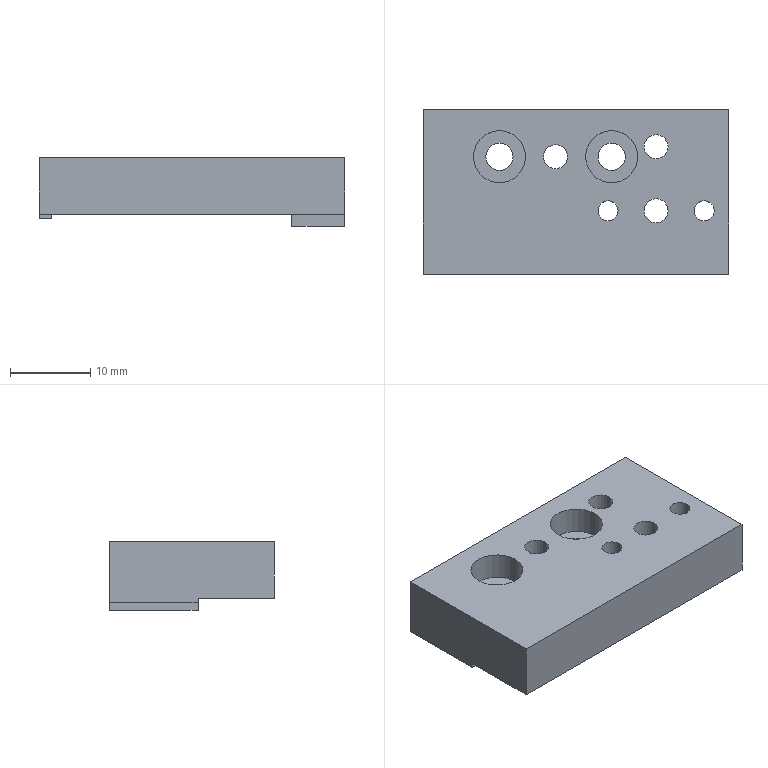Part | STEP file | 11-FG-E02711 | 1 solid | 32 faces | box 38.1 x 20.5 x 8.5 mm | volume 5078 mm3 | cylinder 18 | plane 14 | commonest cylinder face diameters 3 x6 2.5 x4 3.4 x4 6.5 x4
STEP:
#1=CARTESIAN_POINT('',(14.05,8.4,0.));
#2=VERTEX_POINT('',#1);
#3=CARTESIAN_POINT('',(11.05,8.4,0.));
#4=VERTEX_POINT('',#3);
#5=CARTESIAN_POINT('',(12.55,8.4,0.));
#6=DIRECTION('',(0.,0.,-1.));
#7=DIRECTION('',(-1.,0.,0.));
#8=AXIS2_PLACEMENT_3D('',#5,#6,#7);
#9=CIRCLE('',#8,1.5);
#10=EDGE_CURVE('',#2,#4,#9,.T.);
#11=ORIENTED_EDGE('',*,*,#10,.T.);
#12=CARTESIAN_POINT('',(11.05,8.4,7.));
#13=VERTEX_POINT('',#12);
#14=CARTESIAN_POINT('',(11.05,8.4,7.));
#15=DIRECTION('',(0.,0.,1.));
#16=VECTOR('',#15,1000.);
#17=LINE('',#14,#16);
#18=EDGE_CURVE('',#4,#13,#17,.T.);
#19=ORIENTED_EDGE('',*,*,#18,.T.);
#20=CARTESIAN_POINT('',(14.05,8.4,7.));
#21=VERTEX_POINT('',#20);
#22=CARTESIAN_POINT('',(12.55,8.4,7.));
#23=DIRECTION('',(0.,0.,1.));
#24=DIRECTION('',(1.,0.,0.));
#25=AXIS2_PLACEMENT_3D('',#22,#23,#24);
#26=CIRCLE('',#25,1.5);
#27=EDGE_CURVE('',#13,#21,#26,.T.);
#28=ORIENTED_EDGE('',*,*,#27,.T.);
#29=CARTESIAN_POINT('',(14.05,8.4,7.));
#30=DIRECTION('',(0.,0.,1.));
#31=VECTOR('',#30,1000.);
#32=LINE('',#29,#31);
#33=EDGE_CURVE('',#2,#21,#32,.T.);
#34=ORIENTED_EDGE('',*,*,#33,.F.);
#35=EDGE_LOOP('',(#11,#19,#28,#34));
#36=FACE_OUTER_BOUND('',#35,.T.);
#37=CARTESIAN_POINT('',(12.55,8.4,7.));
#38=DIRECTION('',(0.,0.,1.));
#39=DIRECTION('',(1.,0.,0.));
#40=AXIS2_PLACEMENT_3D('',#37,#38,#39);
#41=CYLINDRICAL_SURFACE('',#40,1.5);
#42=ADVANCED_FACE('',(#36),#41,.F.);
#43=CARTESIAN_POINT('',(14.05,16.4,0.));
#44=VERTEX_POINT('',#43);
#45=CARTESIAN_POINT('',(11.05,16.4,0.));
#46=VERTEX_POINT('',#45);
#47=CARTESIAN_POINT('',(12.55,16.4,0.));
#48=DIRECTION('',(0.,0.,-1.));
#49=DIRECTION('',(-1.,0.,0.));
#50=AXIS2_PLACEMENT_3D('',#47,#48,#49);
#51=CIRCLE('',#50,1.5);
#52=EDGE_CURVE('',#44,#46,#51,.T.);
#53=ORIENTED_EDGE('',*,*,#52,.T.);
#54=CARTESIAN_POINT('',(11.05,16.4,7.));
#55=VERTEX_POINT('',#54);
#56=CARTESIAN_POINT('',(11.05,16.4,7.));
#57=DIRECTION('',(0.,0.,1.));
#58=VECTOR('',#57,1000.);
#59=LINE('',#56,#58);
#60=EDGE_CURVE('',#46,#55,#59,.T.);
#61=ORIENTED_EDGE('',*,*,#60,.T.);
#62=CARTESIAN_POINT('',(14.05,16.4,7.));
#63=VERTEX_POINT('',#62);
#64=CARTESIAN_POINT('',(12.55,16.4,7.));
#65=DIRECTION('',(0.,0.,1.));
#66=DIRECTION('',(1.,0.,0.));
#67=AXIS2_PLACEMENT_3D('',#64,#65,#66);
#68=CIRCLE('',#67,1.5);
#69=EDGE_CURVE('',#55,#63,#68,.T.);
#70=ORIENTED_EDGE('',*,*,#69,.T.);
#71=CARTESIAN_POINT('',(14.05,16.4,7.));
#72=DIRECTION('',(0.,0.,1.));
#73=VECTOR('',#72,1000.);
#74=LINE('',#71,#73);
#75=EDGE_CURVE('',#44,#63,#74,.T.);
#76=ORIENTED_EDGE('',*,*,#75,.F.);
#77=EDGE_LOOP('',(#53,#61,#70,#76));
#78=FACE_OUTER_BOUND('',#77,.T.);
#79=CARTESIAN_POINT('',(12.55,16.4,7.));
#80=DIRECTION('',(0.,0.,1.));
#81=DIRECTION('',(1.,0.,0.));
#82=AXIS2_PLACEMENT_3D('',#79,#80,#81);
#83=CYLINDRICAL_SURFACE('',#82,1.5);
#84=ADVANCED_FACE('',(#78),#83,.F.);
#85=CARTESIAN_POINT('',(-1.5,15.147,0.));
#86=VERTEX_POINT('',#85);
#87=CARTESIAN_POINT('',(1.5,15.147,0.));
#88=VERTEX_POINT('',#87);
#89=CARTESIAN_POINT('',(0.,15.147,0.));
#90=DIRECTION('',(0.,0.,1.));
#91=DIRECTION('',(1.,0.,0.));
#92=AXIS2_PLACEMENT_3D('',#89,#90,#91);
#93=CIRCLE('',#92,1.5);
#94=EDGE_CURVE('',#86,#88,#93,.T.);
#95=ORIENTED_EDGE('',*,*,#94,.F.);
#96=CARTESIAN_POINT('',(-1.5,15.147,7.));
#97=VERTEX_POINT('',#96);
#98=CARTESIAN_POINT('',(-1.5,15.147,7.));
#99=DIRECTION('',(0.,0.,1.));
#100=VECTOR('',#99,1000.);
#101=LINE('',#98,#100);
#102=EDGE_CURVE('',#86,#97,#101,.T.);
#103=ORIENTED_EDGE('',*,*,#102,.T.);
#104=CARTESIAN_POINT('',(1.5,15.147,7.));
#105=VERTEX_POINT('',#104);
#106=CARTESIAN_POINT('',(0.,15.147,7.));
#107=DIRECTION('',(0.,0.,1.));
#108=DIRECTION('',(1.,0.,0.));
#109=AXIS2_PLACEMENT_3D('',#106,#107,#108);
#110=CIRCLE('',#109,1.5);
#111=EDGE_CURVE('',#97,#105,#110,.T.);
#112=ORIENTED_EDGE('',*,*,#111,.T.);
#113=CARTESIAN_POINT('',(1.5,15.147,7.));
#114=DIRECTION('',(0.,0.,1.));
#115=VECTOR('',#114,1000.);
#116=LINE('',#113,#115);
#117=EDGE_CURVE('',#88,#105,#116,.T.);
#118=ORIENTED_EDGE('',*,*,#117,.F.);
#119=EDGE_LOOP('',(#95,#103,#112,#118));
#120=FACE_OUTER_BOUND('',#119,.T.);
#121=CARTESIAN_POINT('',(0.,15.147,7.));
#122=DIRECTION('',(0.,0.,1.));
#123=DIRECTION('',(1.,0.,0.));
#124=AXIS2_PLACEMENT_3D('',#121,#122,#123);
#125=CYLINDRICAL_SURFACE('',#124,1.5);
#126=ADVANCED_FACE('',(#120),#125,.F.);
#127=CARTESIAN_POINT('',(-10.25,15.147,3.6));
#128=VERTEX_POINT('',#127);
#129=CARTESIAN_POINT('',(-3.75,15.147,3.6));
#130=VERTEX_POINT('',#129);
#131=CARTESIAN_POINT('',(-7.,15.147,3.6));
#132=DIRECTION('',(0.,0.,1.));
#133=DIRECTION('',(1.,0.,0.));
#134=AXIS2_PLACEMENT_3D('',#131,#132,#133);
#135=CIRCLE('',#134,3.25);
#136=EDGE_CURVE('',#128,#130,#135,.T.);
#137=ORIENTED_EDGE('',*,*,#136,.F.);
#138=CARTESIAN_POINT('',(-10.25,15.147,7.));
#139=VERTEX_POINT('',#138);
#140=CARTESIAN_POINT('',(-10.25,15.147,7.));
#141=DIRECTION('',(0.,0.,1.));
#142=VECTOR('',#141,1000.);
#143=LINE('',#140,#142);
#144=EDGE_CURVE('',#128,#139,#143,.T.);
#145=ORIENTED_EDGE('',*,*,#144,.T.);
#146=CARTESIAN_POINT('',(-3.75,15.147,7.));
#147=VERTEX_POINT('',#146);
#148=CARTESIAN_POINT('',(-7.,15.147,7.));
#149=DIRECTION('',(0.,0.,1.));
#150=DIRECTION('',(1.,0.,0.));
#151=AXIS2_PLACEMENT_3D('',#148,#149,#150);
#152=CIRCLE('',#151,3.25);
#153=EDGE_CURVE('',#139,#147,#152,.T.);
#154=ORIENTED_EDGE('',*,*,#153,.T.);
#155=CARTESIAN_POINT('',(-3.75,15.147,7.));
#156=DIRECTION('',(0.,0.,1.));
#157=VECTOR('',#156,1000.);
#158=LINE('',#155,#157);
#159=EDGE_CURVE('',#130,#147,#158,.T.);
#160=ORIENTED_EDGE('',*,*,#159,.F.);
#161=EDGE_LOOP('',(#137,#145,#154,#160));
#162=FACE_OUTER_BOUND('',#161,.T.);
#163=CARTESIAN_POINT('',(-7.,15.147,7.));
#164=DIRECTION('',(0.,0.,1.));
#165=DIRECTION('',(1.,0.,0.));
#166=AXIS2_PLACEMENT_3D('',#163,#164,#165);
#167=CYLINDRICAL_SURFACE('',#166,3.25);
#168=ADVANCED_FACE('',(#162),#167,.F.);
#169=CARTESIAN_POINT('',(-8.7,15.147,0.));
#170=VERTEX_POINT('',#169);
#171=CARTESIAN_POINT('',(-5.3,15.147,0.));
#172=VERTEX_POINT('',#171);
#173=CARTESIAN_POINT('',(-7.,15.147,0.));
#174=DIRECTION('',(0.,0.,1.));
#175=DIRECTION('',(1.,0.,0.));
#176=AXIS2_PLACEMENT_3D('',#173,#174,#175);
#177=CIRCLE('',#176,1.7);
#178=EDGE_CURVE('',#170,#172,#177,.T.);
#179=ORIENTED_EDGE('',*,*,#178,.F.);
#180=CARTESIAN_POINT('',(-8.7,15.147,3.6));
#181=VERTEX_POINT('',#180);
#182=CARTESIAN_POINT('',(-8.7,15.147,7.));
#183=DIRECTION('',(0.,0.,1.));
#184=VECTOR('',#183,1000.);
#185=LINE('',#182,#184);
#186=EDGE_CURVE('',#170,#181,#185,.T.);
#187=ORIENTED_EDGE('',*,*,#186,.T.);
#188=CARTESIAN_POINT('',(-5.3,15.147,3.6));
#189=VERTEX_POINT('',#188);
#190=CARTESIAN_POINT('',(-7.,15.147,3.6));
#191=DIRECTION('',(0.,0.,1.));
#192=DIRECTION('',(1.,0.,0.));
#193=AXIS2_PLACEMENT_3D('',#190,#191,#192);
#194=CIRCLE('',#193,1.7);
#195=EDGE_CURVE('',#181,#189,#194,.T.);
#196=ORIENTED_EDGE('',*,*,#195,.T.);
#197=CARTESIAN_POINT('',(-5.3,15.147,7.));
#198=DIRECTION('',(0.,0.,1.));
#199=VECTOR('',#198,1000.);
#200=LINE('',#197,#199);
#201=EDGE_CURVE('',#172,#189,#200,.T.);
#202=ORIENTED_EDGE('',*,*,#201,.F.);
#203=EDGE_LOOP('',(#179,#187,#196,#202));
#204=FACE_OUTER_BOUND('',#203,.T.);
#205=CARTESIAN_POINT('',(-7.,15.147,7.));
#206=DIRECTION('',(0.,0.,1.));
#207=DIRECTION('',(1.,0.,0.));
#208=AXIS2_PLACEMENT_3D('',#205,#206,#207);
#209=CYLINDRICAL_SURFACE('',#208,1.7);
#210=ADVANCED_FACE('',(#204),#209,.F.);
#211=CARTESIAN_POINT('',(3.75,15.147,3.6));
#212=VERTEX_POINT('',#211);
#213=CARTESIAN_POINT('',(10.25,15.147,3.6));
#214=VERTEX_POINT('',#213);
#215=CARTESIAN_POINT('',(7.,15.147,3.6));
#216=DIRECTION('',(0.,0.,1.));
#217=DIRECTION('',(1.,0.,0.));
#218=AXIS2_PLACEMENT_3D('',#215,#216,#217);
#219=CIRCLE('',#218,3.25);
#220=EDGE_CURVE('',#212,#214,#219,.T.);
#221=ORIENTED_EDGE('',*,*,#220,.F.);
#222=CARTESIAN_POINT('',(3.75,15.147,7.));
#223=VERTEX_POINT('',#222);
#224=CARTESIAN_POINT('',(3.75,15.147,7.));
#225=DIRECTION('',(0.,0.,1.));
#226=VECTOR('',#225,1000.);
#227=LINE('',#224,#226);
#228=EDGE_CURVE('',#212,#223,#227,.T.);
#229=ORIENTED_EDGE('',*,*,#228,.T.);
#230=CARTESIAN_POINT('',(10.25,15.147,7.));
#231=VERTEX_POINT('',#230);
#232=CARTESIAN_POINT('',(7.,15.147,7.));
#233=DIRECTION('',(0.,0.,1.));
#234=DIRECTION('',(1.,0.,0.));
#235=AXIS2_PLACEMENT_3D('',#232,#233,#234);
#236=CIRCLE('',#235,3.25);
#237=EDGE_CURVE('',#223,#231,#236,.T.);
#238=ORIENTED_EDGE('',*,*,#237,.T.);
#239=CARTESIAN_POINT('',(10.25,15.147,7.));
#240=DIRECTION('',(0.,0.,1.));
#241=VECTOR('',#240,1000.);
#242=LINE('',#239,#241);
#243=EDGE_CURVE('',#214,#231,#242,.T.);
#244=ORIENTED_EDGE('',*,*,#243,.F.);
#245=EDGE_LOOP('',(#221,#229,#238,#244));
#246=FACE_OUTER_BOUND('',#245,.T.);
#247=CARTESIAN_POINT('',(7.,15.147,7.));
#248=DIRECTION('',(0.,0.,1.));
#249=DIRECTION('',(1.,0.,0.));
#250=AXIS2_PLACEMENT_3D('',#247,#248,#249);
#251=CYLINDRICAL_SURFACE('',#250,3.25);
#252=ADVANCED_FACE('',(#246),#251,.F.);
#253=CARTESIAN_POINT('',(5.3,15.147,0.));
#254=VERTEX_POINT('',#253);
#255=CARTESIAN_POINT('',(8.7,15.147,0.));
#256=VERTEX_POINT('',#255);
#257=CARTESIAN_POINT('',(7.,15.147,0.));
#258=DIRECTION('',(0.,0.,1.));
#259=DIRECTION('',(1.,0.,0.));
#260=AXIS2_PLACEMENT_3D('',#257,#258,#259);
#261=CIRCLE('',#260,1.7);
#262=EDGE_CURVE('',#254,#256,#261,.T.);
#263=ORIENTED_EDGE('',*,*,#262,.F.);
#264=CARTESIAN_POINT('',(5.3,15.147,3.6));
#265=VERTEX_POINT('',#264);
#266=CARTESIAN_POINT('',(5.3,15.147,7.));
#267=DIRECTION('',(0.,0.,1.));
#268=VECTOR('',#267,1000.);
#269=LINE('',#266,#268);
#270=EDGE_CURVE('',#254,#265,#269,.T.);
#271=ORIENTED_EDGE('',*,*,#270,.T.);
#272=CARTESIAN_POINT('',(8.7,15.147,3.6));
#273=VERTEX_POINT('',#272);
#274=CARTESIAN_POINT('',(7.,15.147,3.6));
#275=DIRECTION('',(0.,0.,1.));
#276=DIRECTION('',(1.,0.,0.));
#277=AXIS2_PLACEMENT_3D('',#274,#275,#276);
#278=CIRCLE('',#277,1.7);
#279=EDGE_CURVE('',#265,#273,#278,.T.);
#280=ORIENTED_EDGE('',*,*,#279,.T.);
#281=CARTESIAN_POINT('',(8.7,15.147,7.));
#282=DIRECTION('',(0.,0.,1.));
#283=VECTOR('',#282,1000.);
#284=LINE('',#281,#283);
#285=EDGE_CURVE('',#256,#273,#284,.T.);
#286=ORIENTED_EDGE('',*,*,#285,.F.);
#287=EDGE_LOOP('',(#263,#271,#280,#286));
#288=FACE_OUTER_BOUND('',#287,.T.);
#289=CARTESIAN_POINT('',(7.,15.147,7.));
#290=DIRECTION('',(0.,0.,1.));
#291=DIRECTION('',(1.,0.,0.));
#292=AXIS2_PLACEMENT_3D('',#289,#290,#291);
#293=CYLINDRICAL_SURFACE('',#292,1.7);
#294=ADVANCED_FACE('',(#288),#293,.F.);
#295=CARTESIAN_POINT('',(5.3,8.4,0.));
#296=VERTEX_POINT('',#295);
#297=CARTESIAN_POINT('',(7.8,8.4,0.));
#298=VERTEX_POINT('',#297);
#299=CARTESIAN_POINT('',(6.55,8.4,0.));
#300=DIRECTION('',(0.,0.,1.));
#301=DIRECTION('',(1.,0.,0.));
#302=AXIS2_PLACEMENT_3D('',#299,#300,#301);
#303=CIRCLE('',#302,1.25);
#304=EDGE_CURVE('',#296,#298,#303,.T.);
#305=ORIENTED_EDGE('',*,*,#304,.F.);
#306=CARTESIAN_POINT('',(5.3,8.4,7.));
#307=VERTEX_POINT('',#306);
#308=CARTESIAN_POINT('',(5.3,8.4,7.));
#309=DIRECTION('',(0.,0.,1.));
#310=VECTOR('',#309,1000.);
#311=LINE('',#308,#310);
#312=EDGE_CURVE('',#296,#307,#311,.T.);
#313=ORIENTED_EDGE('',*,*,#312,.T.);
#314=CARTESIAN_POINT('',(7.8,8.4,7.));
#315=VERTEX_POINT('',#314);
#316=CARTESIAN_POINT('',(6.55,8.4,7.));
#317=DIRECTION('',(0.,0.,1.));
#318=DIRECTION('',(1.,0.,0.));
#319=AXIS2_PLACEMENT_3D('',#316,#317,#318);
#320=CIRCLE('',#319,1.25);
#321=EDGE_CURVE('',#307,#315,#320,.T.);
#322=ORIENTED_EDGE('',*,*,#321,.T.);
#323=CARTESIAN_POINT('',(7.8,8.4,7.));
#324=DIRECTION('',(0.,0.,1.));
#325=VECTOR('',#324,1000.);
#326=LINE('',#323,#325);
#327=EDGE_CURVE('',#298,#315,#326,.T.);
#328=ORIENTED_EDGE('',*,*,#327,.F.);
#329=EDGE_LOOP('',(#305,#313,#322,#328));
#330=FACE_OUTER_BOUND('',#329,.T.);
#331=CARTESIAN_POINT('',(6.55,8.4,7.));
#332=DIRECTION('',(0.,0.,1.));
#333=DIRECTION('',(1.,0.,0.));
#334=AXIS2_PLACEMENT_3D('',#331,#332,#333);
#335=CYLINDRICAL_SURFACE('',#334,1.25);
#336=ADVANCED_FACE('',(#330),#335,.F.);
#337=CARTESIAN_POINT('',(17.3,8.4,0.));
#338=VERTEX_POINT('',#337);
#339=CARTESIAN_POINT('',(19.8,8.4,0.));
#340=VERTEX_POINT('',#339);
#341=CARTESIAN_POINT('',(18.55,8.4,0.));
#342=DIRECTION('',(0.,0.,1.));
#343=DIRECTION('',(1.,0.,0.));
#344=AXIS2_PLACEMENT_3D('',#341,#342,#343);
#345=CIRCLE('',#344,1.25);
#346=EDGE_CURVE('',#338,#340,#345,.T.);
#347=ORIENTED_EDGE('',*,*,#346,.F.);
#348=CARTESIAN_POINT('',(17.3,8.4,7.));
#349=VERTEX_POINT('',#348);
#350=CARTESIAN_POINT('',(17.3,8.4,7.));
#351=DIRECTION('',(0.,0.,1.));
#352=VECTOR('',#351,1000.);
#353=LINE('',#350,#352);
#354=EDGE_CURVE('',#338,#349,#353,.T.);
#355=ORIENTED_EDGE('',*,*,#354,.T.);
#356=CARTESIAN_POINT('',(19.8,8.4,7.));
#357=VERTEX_POINT('',#356);
#358=CARTESIAN_POINT('',(18.55,8.4,7.));
#359=DIRECTION('',(0.,0.,1.));
#360=DIRECTION('',(1.,0.,0.));
#361=AXIS2_PLACEMENT_3D('',#358,#359,#360);
#362=CIRCLE('',#361,1.25);
#363=EDGE_CURVE('',#349,#357,#362,.T.);
#364=ORIENTED_EDGE('',*,*,#363,.T.);
#365=CARTESIAN_POINT('',(19.8,8.4,7.));
#366=DIRECTION('',(0.,0.,1.));
#367=VECTOR('',#366,1000.);
#368=LINE('',#365,#367);
#369=EDGE_CURVE('',#340,#357,#368,.T.);
#370=ORIENTED_EDGE('',*,*,#369,.F.);
#371=EDGE_LOOP('',(#347,#355,#364,#370));
#372=FACE_OUTER_BOUND('',#371,.T.);
#373=CARTESIAN_POINT('',(18.55,8.4,7.));
#374=DIRECTION('',(0.,0.,1.));
#375=DIRECTION('',(1.,0.,0.));
#376=AXIS2_PLACEMENT_3D('',#373,#374,#375);
#377=CYLINDRICAL_SURFACE('',#376,1.25);
#378=ADVANCED_FACE('',(#372),#377,.F.);
#379=CARTESIAN_POINT('',(-16.5,10.,0.));
#380=VERTEX_POINT('',#379);
#381=CARTESIAN_POINT('',(-16.5,0.5,0.));
#382=VERTEX_POINT('',#381);
#383=CARTESIAN_POINT('',(-16.5,0.,0.));
#384=DIRECTION('',(0.,-1.,0.));
#385=VECTOR('',#384,1000.);
#386=LINE('',#383,#385);
#387=EDGE_CURVE('',#380,#382,#386,.T.);
#388=ORIENTED_EDGE('',*,*,#387,.F.);
#389=CARTESIAN_POINT('',(-15.,10.,0.));
#390=VERTEX_POINT('',#389);
#391=CARTESIAN_POINT('',(-23.4,10.,0.));
#392=DIRECTION('',(-1.,0.,0.));
#393=VECTOR('',#392,1000.);
#394=LINE('',#391,#393);
#395=EDGE_CURVE('',#390,#380,#394,.T.);
#396=ORIENTED_EDGE('',*,*,#395,.F.);
#397=CARTESIAN_POINT('',(-15.,21.,0.));
#398=VERTEX_POINT('',#397);
#399=CARTESIAN_POINT('',(-15.,21.,0.));
#400=DIRECTION('',(0.,-1.,0.));
#401=VECTOR('',#400,1000.);
#402=LINE('',#399,#401);
#403=EDGE_CURVE('',#398,#390,#402,.T.);
#404=ORIENTED_EDGE('',*,*,#403,.F.);
#405=CARTESIAN_POINT('',(15.,21.,0.));
#406=VERTEX_POINT('',#405);
#407=CARTESIAN_POINT('',(-27.5,21.,0.));
#408=DIRECTION('',(-1.,0.,0.));
#409=VECTOR('',#408,1000.);
#410=LINE('',#407,#409);
#411=EDGE_CURVE('',#406,#398,#410,.T.);
#412=ORIENTED_EDGE('',*,*,#411,.F.);
#413=CARTESIAN_POINT('',(15.,10.,0.));
#414=VERTEX_POINT('',#413);
#415=CARTESIAN_POINT('',(15.,10.,0.));
#416=DIRECTION('',(0.,1.,0.));
#417=VECTOR('',#416,1000.);
#418=LINE('',#415,#417);
#419=EDGE_CURVE('',#414,#406,#418,.T.);
#420=ORIENTED_EDGE('',*,*,#419,.F.);
#421=CARTESIAN_POINT('',(21.6,10.,0.));
#422=VERTEX_POINT('',#421);
#423=CARTESIAN_POINT('',(21.6,10.,0.));
#424=DIRECTION('',(-1.,0.,0.));
#425=VECTOR('',#424,1000.);
#426=LINE('',#423,#425);
#427=EDGE_CURVE('',#422,#414,#426,.T.);
#428=ORIENTED_EDGE('',*,*,#427,.F.);
#429=CARTESIAN_POINT('',(21.6,0.5,0.));
#430=VERTEX_POINT('',#429);
#431=CARTESIAN_POINT('',(21.6,0.,0.));
#432=DIRECTION('',(0.,1.,0.));
#433=VECTOR('',#432,1000.);
#434=LINE('',#431,#433);
#435=EDGE_CURVE('',#430,#422,#434,.T.);
#436=ORIENTED_EDGE('',*,*,#435,.F.);
#437=CARTESIAN_POINT('',(0.,0.5,0.));
#438=DIRECTION('',(1.,0.,0.));
#439=VECTOR('',#438,1000.);
#440=LINE('',#437,#439);
#441=EDGE_CURVE('',#382,#430,#440,.T.);
#442=ORIENTED_EDGE('',*,*,#441,.F.);
#443=EDGE_LOOP('',(#388,#396,#404,#412,#420,#428,#436,#442));
#444=FACE_OUTER_BOUND('',#443,.T.);
#445=ORIENTED_EDGE('',*,*,#10,.F.);
#446=CARTESIAN_POINT('',(12.55,8.4,0.));
#447=DIRECTION('',(0.,0.,-1.));
#448=DIRECTION('',(-1.,0.,0.));
#449=AXIS2_PLACEMENT_3D('',#446,#447,#448);
#450=CIRCLE('',#449,1.5);
#451=EDGE_CURVE('',#4,#2,#450,.T.);
#452=ORIENTED_EDGE('',*,*,#451,.F.);
#453=EDGE_LOOP('',(#445,#452));
#454=FACE_BOUND('',#453,.T.);
#455=ORIENTED_EDGE('',*,*,#52,.F.);
#456=CARTESIAN_POINT('',(12.55,16.4,0.));
#457=DIRECTION('',(0.,0.,-1.));
#458=DIRECTION('',(-1.,0.,0.));
#459=AXIS2_PLACEMENT_3D('',#456,#457,#458);
#460=CIRCLE('',#459,1.5);
#461=EDGE_CURVE('',#46,#44,#460,.T.);
#462=ORIENTED_EDGE('',*,*,#461,.F.);
#463=EDGE_LOOP('',(#455,#462));
#464=FACE_BOUND('',#463,.T.);
#465=CARTESIAN_POINT('',(0.,15.147,0.));
#466=DIRECTION('',(0.,0.,1.));
#467=DIRECTION('',(1.,0.,0.));
#468=AXIS2_PLACEMENT_3D('',#465,#466,#467);
#469=CIRCLE('',#468,1.5);
#470=EDGE_CURVE('',#88,#86,#469,.T.);
#471=ORIENTED_EDGE('',*,*,#470,.T.);
#472=ORIENTED_EDGE('',*,*,#94,.T.);
#473=EDGE_LOOP('',(#471,#472));
#474=FACE_BOUND('',#473,.T.);
#475=CARTESIAN_POINT('',(-7.,15.147,0.));
#476=DIRECTION('',(0.,0.,1.));
#477=DIRECTION('',(1.,0.,0.));
#478=AXIS2_PLACEMENT_3D('',#475,#476,#477);
#479=CIRCLE('',#478,1.7);
#480=EDGE_CURVE('',#172,#170,#479,.T.);
#481=ORIENTED_EDGE('',*,*,#480,.T.);
#482=ORIENTED_EDGE('',*,*,#178,.T.);
#483=EDGE_LOOP('',(#481,#482));
#484=FACE_BOUND('',#483,.T.);
#485=CARTESIAN_POINT('',(7.,15.147,0.));
#486=DIRECTION('',(0.,0.,1.));
#487=DIRECTION('',(1.,0.,0.));
#488=AXIS2_PLACEMENT_3D('',#485,#486,#487);
#489=CIRCLE('',#488,1.7);
#490=EDGE_CURVE('',#256,#254,#489,.T.);
#491=ORIENTED_EDGE('',*,*,#490,.T.);
#492=ORIENTED_EDGE('',*,*,#262,.T.);
#493=EDGE_LOOP('',(#491,#492));
#494=FACE_BOUND('',#493,.T.);
#495=CARTESIAN_POINT('',(6.55,8.4,0.));
#496=DIRECTION('',(0.,0.,1.));
#497=DIRECTION('',(1.,0.,0.));
#498=AXIS2_PLACEMENT_3D('',#495,#496,#497);
#499=CIRCLE('',#498,1.25);
#500=EDGE_CURVE('',#298,#296,#499,.T.);
#501=ORIENTED_EDGE('',*,*,#500,.T.);
#502=ORIENTED_EDGE('',*,*,#304,.T.);
#503=EDGE_LOOP('',(#501,#502));
#504=FACE_BOUND('',#503,.T.);
#505=CARTESIAN_POINT('',(18.55,8.4,0.));
#506=DIRECTION('',(0.,0.,1.));
#507=DIRECTION('',(1.,0.,0.));
#508=AXIS2_PLACEMENT_3D('',#505,#506,#507);
#509=CIRCLE('',#508,1.25);
#510=EDGE_CURVE('',#340,#338,#509,.T.);
#511=ORIENTED_EDGE('',*,*,#510,.T.);
#512=ORIENTED_EDGE('',*,*,#346,.T.);
#513=EDGE_LOOP('',(#511,#512));
#514=FACE_BOUND('',#513,.T.);
#515=CARTESIAN_POINT('',(0.,0.,0.));
#516=DIRECTION('',(0.,0.,-1.));
#517=DIRECTION('',(-1.,0.,0.));
#518=AXIS2_PLACEMENT_3D('',#515,#516,#517);
#519=PLANE('',#518);
#520=ADVANCED_FACE('',(#444,#454,#464,#474,#484,#494,#504,#514),#519,.T.);
#521=CARTESIAN_POINT('',(-15.,21.,-0.6));
#522=VERTEX_POINT('',#521);
#523=CARTESIAN_POINT('',(-15.,21.,-2.));
#524=DIRECTION('',(0.,0.,1.));
#525=VECTOR('',#524,1000.);
#526=LINE('',#523,#525);
#527=EDGE_CURVE('',#522,#398,#526,.T.);
#528=ORIENTED_EDGE('',*,*,#527,.F.);
#529=CARTESIAN_POINT('',(-16.5,21.,-0.6));
#530=VERTEX_POINT('',#529);
#531=CARTESIAN_POINT('',(-15.,21.,-0.6));
#532=DIRECTION('',(1.,0.,0.));
#533=VECTOR('',#532,1000.);
#534=LINE('',#531,#533);
#535=EDGE_CURVE('',#530,#522,#534,.T.);
#536=ORIENTED_EDGE('',*,*,#535,.F.);
#537=CARTESIAN_POINT('',(-16.5,21.,7.));
#538=VERTEX_POINT('',#537);
#539=CARTESIAN_POINT('',(-16.5,21.,-2.));
#540=DIRECTION('',(0.,0.,-1.));
#541=VECTOR('',#540,1000.);
#542=LINE('',#539,#541);
#543=EDGE_CURVE('',#538,#530,#542,.T.);
#544=ORIENTED_EDGE('',*,*,#543,.F.);
#545=CARTESIAN_POINT('',(21.6,21.,7.));
#546=VERTEX_POINT('',#545);
#547=CARTESIAN_POINT('',(-27.5,21.,7.));
#548=DIRECTION('',(-1.,0.,0.));
#549=VECTOR('',#548,1000.);
#550=LINE('',#547,#549);
#551=EDGE_CURVE('',#546,#538,#550,.T.);
#552=ORIENTED_EDGE('',*,*,#551,.F.);
#553=CARTESIAN_POINT('',(21.6,21.,-1.5));
#554=VERTEX_POINT('',#553);
#555=CARTESIAN_POINT('',(21.6,21.,-3.));
#556=DIRECTION('',(0.,0.,1.));
#557=VECTOR('',#556,1000.);
#558=LINE('',#555,#557);
#559=EDGE_CURVE('',#554,#546,#558,.T.);
#560=ORIENTED_EDGE('',*,*,#559,.F.);
#561=CARTESIAN_POINT('',(15.,21.,-1.5));
#562=VERTEX_POINT('',#561);
#563=CARTESIAN_POINT('',(-16.5,21.,-1.5));
#564=DIRECTION('',(1.,0.,0.));
#565=VECTOR('',#564,1000.);
#566=LINE('',#563,#565);
#567=EDGE_CURVE('',#562,#554,#566,.T.);
#568=ORIENTED_EDGE('',*,*,#567,.F.);
#569=CARTESIAN_POINT('',(15.,21.,-2.));
#570=DIRECTION('',(0.,0.,1.));
#571=VECTOR('',#570,1000.);
#572=LINE('',#569,#571);
#573=EDGE_CURVE('',#562,#406,#572,.T.);
#574=ORIENTED_EDGE('',*,*,#573,.T.);
#575=ORIENTED_EDGE('',*,*,#411,.T.);
#576=EDGE_LOOP('',(#528,#536,#544,#552,#560,#568,#574,#575));
#577=FACE_OUTER_BOUND('',#576,.T.);
#578=CARTESIAN_POINT('',(-27.5,21.,7.));
#579=DIRECTION('',(0.,-1.,0.));
#580=DIRECTION('',(0.,0.,-1.));
#581=AXIS2_PLACEMENT_3D('',#578,#579,#580);
#582=PLANE('',#581);
#583=ADVANCED_FACE('',(#577),#582,.F.);
#584=CARTESIAN_POINT('',(12.55,8.4,7.));
#585=DIRECTION('',(0.,0.,1.));
#586=DIRECTION('',(1.,0.,0.));
#587=AXIS2_PLACEMENT_3D('',#584,#585,#586);
#588=CIRCLE('',#587,1.5);
#589=EDGE_CURVE('',#21,#13,#588,.T.);
#590=ORIENTED_EDGE('',*,*,#589,.F.);
#591=ORIENTED_EDGE('',*,*,#27,.F.);
#592=EDGE_LOOP('',(#590,#591));
#593=FACE_BOUND('',#592,.T.);
#594=CARTESIAN_POINT('',(12.55,16.4,7.));
#595=DIRECTION('',(0.,0.,1.));
#596=DIRECTION('',(1.,0.,0.));
#597=AXIS2_PLACEMENT_3D('',#594,#595,#596);
#598=CIRCLE('',#597,1.5);
#599=EDGE_CURVE('',#63,#55,#598,.T.);
#600=ORIENTED_EDGE('',*,*,#599,.F.);
#601=ORIENTED_EDGE('',*,*,#69,.F.);
#602=EDGE_LOOP('',(#600,#601));
#603=FACE_BOUND('',#602,.T.);
#604=CARTESIAN_POINT('',(0.,15.147,7.));
#605=DIRECTION('',(0.,0.,1.));
#606=DIRECTION('',(1.,0.,0.));
#607=AXIS2_PLACEMENT_3D('',#604,#605,#606);
#608=CIRCLE('',#607,1.5);
#609=EDGE_CURVE('',#105,#97,#608,.T.);
#610=ORIENTED_EDGE('',*,*,#609,.F.);
#611=ORIENTED_EDGE('',*,*,#111,.F.);
#612=EDGE_LOOP('',(#610,#611));
#613=FACE_BOUND('',#612,.T.);
#614=CARTESIAN_POINT('',(-7.,15.147,7.));
#615=DIRECTION('',(0.,0.,1.));
#616=DIRECTION('',(1.,0.,0.));
#617=AXIS2_PLACEMENT_3D('',#614,#615,#616);
#618=CIRCLE('',#617,3.25);
#619=EDGE_CURVE('',#147,#139,#618,.T.);
#620=ORIENTED_EDGE('',*,*,#619,.F.);
#621=ORIENTED_EDGE('',*,*,#153,.F.);
#622=EDGE_LOOP('',(#620,#621));
#623=FACE_BOUND('',#622,.T.);
#624=CARTESIAN_POINT('',(7.,15.147,7.));
#625=DIRECTION('',(0.,0.,1.));
#626=DIRECTION('',(1.,0.,0.));
#627=AXIS2_PLACEMENT_3D('',#624,#625,#626);
#628=CIRCLE('',#627,3.25);
#629=EDGE_CURVE('',#231,#223,#628,.T.);
#630=ORIENTED_EDGE('',*,*,#629,.F.);
#631=ORIENTED_EDGE('',*,*,#237,.F.);
#632=EDGE_LOOP('',(#630,#631));
#633=FACE_BOUND('',#632,.T.);
#634=CARTESIAN_POINT('',(6.55,8.4,7.));
#635=DIRECTION('',(0.,0.,1.));
#636=DIRECTION('',(1.,0.,0.));
#637=AXIS2_PLACEMENT_3D('',#634,#635,#636);
#638=CIRCLE('',#637,1.25);
#639=EDGE_CURVE('',#315,#307,#638,.T.);
#640=ORIENTED_EDGE('',*,*,#639,.F.);
#641=ORIENTED_EDGE('',*,*,#321,.F.);
#642=EDGE_LOOP('',(#640,#641));
#643=FACE_BOUND('',#642,.T.);
#644=CARTESIAN_POINT('',(18.55,8.4,7.));
#645=DIRECTION('',(0.,0.,1.));
#646=DIRECTION('',(1.,0.,0.));
#647=AXIS2_PLACEMENT_3D('',#644,#645,#646);
#648=CIRCLE('',#647,1.25);
#649=EDGE_CURVE('',#357,#349,#648,.T.);
#650=ORIENTED_EDGE('',*,*,#649,.F.);
#651=ORIENTED_EDGE('',*,*,#363,.F.);
#652=EDGE_LOOP('',(#650,#651));
#653=FACE_BOUND('',#652,.T.);
#654=ORIENTED_EDGE('',*,*,#551,.T.);
#655=CARTESIAN_POINT('',(-16.5,0.5,7.));
#656=VERTEX_POINT('',#655);
#657=CARTESIAN_POINT('',(-16.5,-20.,7.));
#658=DIRECTION('',(0.,1.,0.));
#659=VECTOR('',#658,1000.);
#660=LINE('',#657,#659);
#661=EDGE_CURVE('',#656,#538,#660,.T.);
#662=ORIENTED_EDGE('',*,*,#661,.F.);
#663=CARTESIAN_POINT('',(21.6,0.5,7.));
#664=VERTEX_POINT('',#663);
#665=CARTESIAN_POINT('',(27.5,0.5,7.));
#666=DIRECTION('',(-1.,0.,0.));
#667=VECTOR('',#666,1000.);
#668=LINE('',#665,#667);
#669=EDGE_CURVE('',#664,#656,#668,.T.);
#670=ORIENTED_EDGE('',*,*,#669,.F.);
#671=CARTESIAN_POINT('',(21.6,-2.5,7.));
#672=DIRECTION('',(0.,-1.,0.));
#673=VECTOR('',#672,1000.);
#674=LINE('',#671,#673);
#675=EDGE_CURVE('',#546,#664,#674,.T.);
#676=ORIENTED_EDGE('',*,*,#675,.F.);
#677=EDGE_LOOP('',(#654,#662,#670,#676));
#678=FACE_OUTER_BOUND('',#677,.T.);
#679=CARTESIAN_POINT('',(0.,0.,7.));
#680=DIRECTION('',(0.,0.,-1.));
#681=DIRECTION('',(-1.,0.,0.));
#682=AXIS2_PLACEMENT_3D('',#679,#680,#681);
#683=PLANE('',#682);
#684=ADVANCED_FACE('',(#593,#603,#613,#623,#633,#643,#653,#678),#683,.F.);
#685=ORIENTED_EDGE('',*,*,#669,.T.);
#686=CARTESIAN_POINT('',(-16.5,0.5,-3.));
#687=DIRECTION('',(0.,0.,-1.));
#688=VECTOR('',#687,1000.);
#689=LINE('',#686,#688);
#690=EDGE_CURVE('',#656,#382,#689,.T.);
#691=ORIENTED_EDGE('',*,*,#690,.T.);
#692=ORIENTED_EDGE('',*,*,#441,.T.);
#693=CARTESIAN_POINT('',(21.6,0.5,-3.));
#694=DIRECTION('',(0.,0.,1.));
#695=VECTOR('',#694,1000.);
#696=LINE('',#693,#695);
#697=EDGE_CURVE('',#430,#664,#696,.T.);
#698=ORIENTED_EDGE('',*,*,#697,.T.);
#699=EDGE_LOOP('',(#685,#691,#692,#698));
#700=FACE_OUTER_BOUND('',#699,.T.);
#701=CARTESIAN_POINT('',(27.5,0.5,-3.));
#702=DIRECTION('',(0.,1.,0.));
#703=DIRECTION('',(-1.,0.,0.));
#704=AXIS2_PLACEMENT_3D('',#701,#702,#703);
#705=PLANE('',#704);
#706=ADVANCED_FACE('',(#700),#705,.F.);
#707=ORIENTED_EDGE('',*,*,#354,.F.);
#708=ORIENTED_EDGE('',*,*,#510,.F.);
#709=ORIENTED_EDGE('',*,*,#369,.T.);
#710=ORIENTED_EDGE('',*,*,#649,.T.);
#711=EDGE_LOOP('',(#707,#708,#709,#710));
#712=FACE_OUTER_BOUND('',#711,.T.);
#713=CARTESIAN_POINT('',(18.55,8.4,7.));
#714=DIRECTION('',(0.,0.,1.));
#715=DIRECTION('',(1.,0.,0.));
#716=AXIS2_PLACEMENT_3D('',#713,#714,#715);
#717=CYLINDRICAL_SURFACE('',#716,1.25);
#718=ADVANCED_FACE('',(#712),#717,.F.);
#719=ORIENTED_EDGE('',*,*,#312,.F.);
#720=ORIENTED_EDGE('',*,*,#500,.F.);
#721=ORIENTED_EDGE('',*,*,#327,.T.);
#722=ORIENTED_EDGE('',*,*,#639,.T.);
#723=EDGE_LOOP('',(#719,#720,#721,#722));
#724=FACE_OUTER_BOUND('',#723,.T.);
#725=CARTESIAN_POINT('',(6.55,8.4,7.));
#726=DIRECTION('',(0.,0.,1.));
#727=DIRECTION('',(1.,0.,0.));
#728=AXIS2_PLACEMENT_3D('',#725,#726,#727);
#729=CYLINDRICAL_SURFACE('',#728,1.25);
#730=ADVANCED_FACE('',(#724),#729,.F.);
#731=ORIENTED_EDGE('',*,*,#270,.F.);
#732=ORIENTED_EDGE('',*,*,#490,.F.);
#733=ORIENTED_EDGE('',*,*,#285,.T.);
#734=CARTESIAN_POINT('',(7.,15.147,3.6));
#735=DIRECTION('',(0.,0.,1.));
#736=DIRECTION('',(1.,0.,0.));
#737=AXIS2_PLACEMENT_3D('',#734,#735,#736);
#738=CIRCLE('',#737,1.7);
#739=EDGE_CURVE('',#273,#265,#738,.T.);
#740=ORIENTED_EDGE('',*,*,#739,.T.);
#741=EDGE_LOOP('',(#731,#732,#733,#740));
#742=FACE_OUTER_BOUND('',#741,.T.);
#743=CARTESIAN_POINT('',(7.,15.147,7.));
#744=DIRECTION('',(0.,0.,1.));
#745=DIRECTION('',(1.,0.,0.));
#746=AXIS2_PLACEMENT_3D('',#743,#744,#745);
#747=CYLINDRICAL_SURFACE('',#746,1.7);
#748=ADVANCED_FACE('',(#742),#747,.F.);
#749=ORIENTED_EDGE('',*,*,#739,.F.);
#750=ORIENTED_EDGE('',*,*,#279,.F.);
#751=EDGE_LOOP('',(#749,#750));
#752=FACE_BOUND('',#751,.T.);
#753=CARTESIAN_POINT('',(7.,15.147,3.6));
#754=DIRECTION('',(0.,0.,1.));
#755=DIRECTION('',(1.,0.,0.));
#756=AXIS2_PLACEMENT_3D('',#753,#754,#755);
#757=CIRCLE('',#756,3.25);
#758=EDGE_CURVE('',#214,#212,#757,.T.);
#759=ORIENTED_EDGE('',*,*,#758,.T.);
#760=ORIENTED_EDGE('',*,*,#220,.T.);
#761=EDGE_LOOP('',(#759,#760));
#762=FACE_OUTER_BOUND('',#761,.T.);
#763=CARTESIAN_POINT('',(8.7,15.147,3.6));
#764=DIRECTION('',(0.,0.,-1.));
#765=DIRECTION('',(-1.,0.,0.));
#766=AXIS2_PLACEMENT_3D('',#763,#764,#765);
#767=PLANE('',#766);
#768=ADVANCED_FACE('',(#752,#762),#767,.F.);
#769=ORIENTED_EDGE('',*,*,#228,.F.);
#770=ORIENTED_EDGE('',*,*,#758,.F.);
#771=ORIENTED_EDGE('',*,*,#243,.T.);
#772=ORIENTED_EDGE('',*,*,#629,.T.);
#773=EDGE_LOOP('',(#769,#770,#771,#772));
#774=FACE_OUTER_BOUND('',#773,.T.);
#775=CARTESIAN_POINT('',(7.,15.147,7.));
#776=DIRECTION('',(0.,0.,1.));
#777=DIRECTION('',(1.,0.,0.));
#778=AXIS2_PLACEMENT_3D('',#775,#776,#777);
#779=CYLINDRICAL_SURFACE('',#778,3.25);
#780=ADVANCED_FACE('',(#774),#779,.F.);
#781=ORIENTED_EDGE('',*,*,#186,.F.);
#782=ORIENTED_EDGE('',*,*,#480,.F.);
#783=ORIENTED_EDGE('',*,*,#201,.T.);
#784=CARTESIAN_POINT('',(-7.,15.147,3.6));
#785=DIRECTION('',(0.,0.,1.));
#786=DIRECTION('',(1.,0.,0.));
#787=AXIS2_PLACEMENT_3D('',#784,#785,#786);
#788=CIRCLE('',#787,1.7);
#789=EDGE_CURVE('',#189,#181,#788,.T.);
#790=ORIENTED_EDGE('',*,*,#789,.T.);
#791=EDGE_LOOP('',(#781,#782,#783,#790));
#792=FACE_OUTER_BOUND('',#791,.T.);
#793=CARTESIAN_POINT('',(-7.,15.147,7.));
#794=DIRECTION('',(0.,0.,1.));
#795=DIRECTION('',(1.,0.,0.));
#796=AXIS2_PLACEMENT_3D('',#793,#794,#795);
#797=CYLINDRICAL_SURFACE('',#796,1.7);
#798=ADVANCED_FACE('',(#792),#797,.F.);
#799=ORIENTED_EDGE('',*,*,#789,.F.);
#800=ORIENTED_EDGE('',*,*,#195,.F.);
#801=EDGE_LOOP('',(#799,#800));
#802=FACE_BOUND('',#801,.T.);
#803=CARTESIAN_POINT('',(-7.,15.147,3.6));
#804=DIRECTION('',(0.,0.,1.));
#805=DIRECTION('',(1.,0.,0.));
#806=AXIS2_PLACEMENT_3D('',#803,#804,#805);
#807=CIRCLE('',#806,3.25);
#808=EDGE_CURVE('',#130,#128,#807,.T.);
#809=ORIENTED_EDGE('',*,*,#808,.T.);
#810=ORIENTED_EDGE('',*,*,#136,.T.);
#811=EDGE_LOOP('',(#809,#810));
#812=FACE_OUTER_BOUND('',#811,.T.);
#813=CARTESIAN_POINT('',(-5.3,15.147,3.6));
#814=DIRECTION('',(0.,0.,-1.));
#815=DIRECTION('',(-1.,0.,0.));
#816=AXIS2_PLACEMENT_3D('',#813,#814,#815);
#817=PLANE('',#816);
#818=ADVANCED_FACE('',(#802,#812),#817,.F.);
#819=ORIENTED_EDGE('',*,*,#144,.F.);
#820=ORIENTED_EDGE('',*,*,#808,.F.);
#821=ORIENTED_EDGE('',*,*,#159,.T.);
#822=ORIENTED_EDGE('',*,*,#619,.T.);
#823=EDGE_LOOP('',(#819,#820,#821,#822));
#824=FACE_OUTER_BOUND('',#823,.T.);
#825=CARTESIAN_POINT('',(-7.,15.147,7.));
#826=DIRECTION('',(0.,0.,1.));
#827=DIRECTION('',(1.,0.,0.));
#828=AXIS2_PLACEMENT_3D('',#825,#826,#827);
#829=CYLINDRICAL_SURFACE('',#828,3.25);
#830=ADVANCED_FACE('',(#824),#829,.F.);
#831=ORIENTED_EDGE('',*,*,#102,.F.);
#832=ORIENTED_EDGE('',*,*,#470,.F.);
#833=ORIENTED_EDGE('',*,*,#117,.T.);
#834=ORIENTED_EDGE('',*,*,#609,.T.);
#835=EDGE_LOOP('',(#831,#832,#833,#834));
#836=FACE_OUTER_BOUND('',#835,.T.);
#837=CARTESIAN_POINT('',(0.,15.147,7.));
#838=DIRECTION('',(0.,0.,1.));
#839=DIRECTION('',(1.,0.,0.));
#840=AXIS2_PLACEMENT_3D('',#837,#838,#839);
#841=CYLINDRICAL_SURFACE('',#840,1.5);
#842=ADVANCED_FACE('',(#836),#841,.F.);
#843=ORIENTED_EDGE('',*,*,#60,.F.);
#844=ORIENTED_EDGE('',*,*,#461,.T.);
#845=ORIENTED_EDGE('',*,*,#75,.T.);
#846=ORIENTED_EDGE('',*,*,#599,.T.);
#847=EDGE_LOOP('',(#843,#844,#845,#846));
#848=FACE_OUTER_BOUND('',#847,.T.);
#849=CARTESIAN_POINT('',(12.55,16.4,7.));
#850=DIRECTION('',(0.,0.,1.));
#851=DIRECTION('',(1.,0.,0.));
#852=AXIS2_PLACEMENT_3D('',#849,#850,#851);
#853=CYLINDRICAL_SURFACE('',#852,1.5);
#854=ADVANCED_FACE('',(#848),#853,.F.);
#855=ORIENTED_EDGE('',*,*,#18,.F.);
#856=ORIENTED_EDGE('',*,*,#451,.T.);
#857=ORIENTED_EDGE('',*,*,#33,.T.);
#858=ORIENTED_EDGE('',*,*,#589,.T.);
#859=EDGE_LOOP('',(#855,#856,#857,#858));
#860=FACE_OUTER_BOUND('',#859,.T.);
#861=CARTESIAN_POINT('',(12.55,8.4,7.));
#862=DIRECTION('',(0.,0.,1.));
#863=DIRECTION('',(1.,0.,0.));
#864=AXIS2_PLACEMENT_3D('',#861,#862,#863);
#865=CYLINDRICAL_SURFACE('',#864,1.5);
#866=ADVANCED_FACE('',(#860),#865,.F.);
#867=CARTESIAN_POINT('',(21.6,10.,-1.5));
#868=VERTEX_POINT('',#867);
#869=CARTESIAN_POINT('',(21.6,10.,-2.));
#870=DIRECTION('',(0.,0.,1.));
#871=VECTOR('',#870,1000.);
#872=LINE('',#869,#871);
#873=EDGE_CURVE('',#868,#422,#872,.T.);
#874=ORIENTED_EDGE('',*,*,#873,.F.);
#875=CARTESIAN_POINT('',(21.6,-20.,-1.5));
#876=DIRECTION('',(0.,1.,0.));
#877=VECTOR('',#876,1000.);
#878=LINE('',#875,#877);
#879=EDGE_CURVE('',#868,#554,#878,.T.);
#880=ORIENTED_EDGE('',*,*,#879,.T.);
#881=ORIENTED_EDGE('',*,*,#559,.T.);
#882=ORIENTED_EDGE('',*,*,#675,.T.);
#883=ORIENTED_EDGE('',*,*,#697,.F.);
#884=ORIENTED_EDGE('',*,*,#435,.T.);
#885=EDGE_LOOP('',(#874,#880,#881,#882,#883,#884));
#886=FACE_OUTER_BOUND('',#885,.T.);
#887=CARTESIAN_POINT('',(21.6,-2.5,-3.));
#888=DIRECTION('',(-1.,0.,0.));
#889=DIRECTION('',(0.,0.,1.));
#890=AXIS2_PLACEMENT_3D('',#887,#888,#889);
#891=PLANE('',#890);
#892=ADVANCED_FACE('',(#886),#891,.F.);
#893=CARTESIAN_POINT('',(15.,10.,-1.5));
#894=VERTEX_POINT('',#893);
#895=CARTESIAN_POINT('',(15.,10.,-2.));
#896=DIRECTION('',(0.,0.,1.));
#897=VECTOR('',#896,1000.);
#898=LINE('',#895,#897);
#899=EDGE_CURVE('',#894,#414,#898,.T.);
#900=ORIENTED_EDGE('',*,*,#899,.F.);
#901=CARTESIAN_POINT('',(21.6,10.,-1.5));
#902=DIRECTION('',(1.,0.,0.));
#903=VECTOR('',#902,1000.);
#904=LINE('',#901,#903);
#905=EDGE_CURVE('',#894,#868,#904,.T.);
#906=ORIENTED_EDGE('',*,*,#905,.T.);
#907=ORIENTED_EDGE('',*,*,#873,.T.);
#908=ORIENTED_EDGE('',*,*,#427,.T.);
#909=EDGE_LOOP('',(#900,#906,#907,#908));
#910=FACE_OUTER_BOUND('',#909,.T.);
#911=CARTESIAN_POINT('',(21.6,10.,-2.));
#912=DIRECTION('',(0.,1.,0.));
#913=DIRECTION('',(0.,0.,1.));
#914=AXIS2_PLACEMENT_3D('',#911,#912,#913);
#915=PLANE('',#914);
#916=ADVANCED_FACE('',(#910),#915,.F.);
#917=ORIENTED_EDGE('',*,*,#573,.F.);
#918=CARTESIAN_POINT('',(15.,10.,-1.5));
#919=DIRECTION('',(0.,-1.,0.));
#920=VECTOR('',#919,1000.);
#921=LINE('',#918,#920);
#922=EDGE_CURVE('',#562,#894,#921,.T.);
#923=ORIENTED_EDGE('',*,*,#922,.T.);
#924=ORIENTED_EDGE('',*,*,#899,.T.);
#925=ORIENTED_EDGE('',*,*,#419,.T.);
#926=EDGE_LOOP('',(#917,#923,#924,#925));
#927=FACE_OUTER_BOUND('',#926,.T.);
#928=CARTESIAN_POINT('',(15.,10.,-2.));
#929=DIRECTION('',(1.,0.,0.));
#930=DIRECTION('',(0.,0.,-1.));
#931=AXIS2_PLACEMENT_3D('',#928,#929,#930);
#932=PLANE('',#931);
#933=ADVANCED_FACE('',(#927),#932,.F.);
#934=CARTESIAN_POINT('',(-15.,10.,-0.6));
#935=VERTEX_POINT('',#934);
#936=CARTESIAN_POINT('',(-15.,10.,-2.));
#937=DIRECTION('',(0.,0.,1.));
#938=VECTOR('',#937,1000.);
#939=LINE('',#936,#938);
#940=EDGE_CURVE('',#935,#390,#939,.T.);
#941=ORIENTED_EDGE('',*,*,#940,.F.);
#942=CARTESIAN_POINT('',(-15.,-20.,-0.6));
#943=DIRECTION('',(0.,1.,0.));
#944=VECTOR('',#943,1000.);
#945=LINE('',#942,#944);
#946=EDGE_CURVE('',#935,#522,#945,.T.);
#947=ORIENTED_EDGE('',*,*,#946,.T.);
#948=ORIENTED_EDGE('',*,*,#527,.T.);
#949=ORIENTED_EDGE('',*,*,#403,.T.);
#950=EDGE_LOOP('',(#941,#947,#948,#949));
#951=FACE_OUTER_BOUND('',#950,.T.);
#952=CARTESIAN_POINT('',(-15.,21.,-2.));
#953=DIRECTION('',(-1.,0.,0.));
#954=DIRECTION('',(0.,-1.,0.));
#955=AXIS2_PLACEMENT_3D('',#952,#953,#954);
#956=PLANE('',#955);
#957=ADVANCED_FACE('',(#951),#956,.F.);
#958=CARTESIAN_POINT('',(-16.5,10.,-0.6));
#959=VERTEX_POINT('',#958);
#960=CARTESIAN_POINT('',(-16.5,10.,-2.));
#961=DIRECTION('',(0.,0.,-1.));
#962=VECTOR('',#961,1000.);
#963=LINE('',#960,#962);
#964=EDGE_CURVE('',#380,#959,#963,.T.);
#965=ORIENTED_EDGE('',*,*,#964,.T.);
#966=CARTESIAN_POINT('',(-23.4,10.,-0.6));
#967=DIRECTION('',(1.,0.,0.));
#968=VECTOR('',#967,1000.);
#969=LINE('',#966,#968);
#970=EDGE_CURVE('',#959,#935,#969,.T.);
#971=ORIENTED_EDGE('',*,*,#970,.T.);
#972=ORIENTED_EDGE('',*,*,#940,.T.);
#973=ORIENTED_EDGE('',*,*,#395,.T.);
#974=EDGE_LOOP('',(#965,#971,#972,#973));
#975=FACE_OUTER_BOUND('',#974,.T.);
#976=CARTESIAN_POINT('',(-23.4,10.,-2.));
#977=DIRECTION('',(0.,1.,0.));
#978=DIRECTION('',(-1.,0.,0.));
#979=AXIS2_PLACEMENT_3D('',#976,#977,#978);
#980=PLANE('',#979);
#981=ADVANCED_FACE('',(#975),#980,.F.);
#982=ORIENTED_EDGE('',*,*,#543,.T.);
#983=CARTESIAN_POINT('',(-16.5,-20.,-0.6));
#984=DIRECTION('',(0.,1.,0.));
#985=VECTOR('',#984,1000.);
#986=LINE('',#983,#985);
#987=EDGE_CURVE('',#959,#530,#986,.T.);
#988=ORIENTED_EDGE('',*,*,#987,.F.);
#989=ORIENTED_EDGE('',*,*,#964,.F.);
#990=ORIENTED_EDGE('',*,*,#387,.T.);
#991=ORIENTED_EDGE('',*,*,#690,.F.);
#992=ORIENTED_EDGE('',*,*,#661,.T.);
#993=EDGE_LOOP('',(#982,#988,#989,#990,#991,#992));
#994=FACE_OUTER_BOUND('',#993,.T.);
#995=CARTESIAN_POINT('',(-16.5,-20.,-2.));
#996=DIRECTION('',(1.,0.,0.));
#997=DIRECTION('',(0.,0.,-1.));
#998=AXIS2_PLACEMENT_3D('',#995,#996,#997);
#999=PLANE('',#998);
#1000=ADVANCED_FACE('',(#994),#999,.F.);
#1001=ORIENTED_EDGE('',*,*,#922,.F.);
#1002=ORIENTED_EDGE('',*,*,#567,.T.);
#1003=ORIENTED_EDGE('',*,*,#879,.F.);
#1004=ORIENTED_EDGE('',*,*,#905,.F.);
#1005=EDGE_LOOP('',(#1001,#1002,#1003,#1004));
#1006=FACE_OUTER_BOUND('',#1005,.T.);
#1007=CARTESIAN_POINT('',(-16.5,-20.,-1.5));
#1008=DIRECTION('',(0.,0.,1.));
#1009=DIRECTION('',(1.,0.,0.));
#1010=AXIS2_PLACEMENT_3D('',#1007,#1008,#1009);
#1011=PLANE('',#1010);
#1012=ADVANCED_FACE('',(#1006),#1011,.F.);
#1013=ORIENTED_EDGE('',*,*,#987,.T.);
#1014=ORIENTED_EDGE('',*,*,#535,.T.);
#1015=ORIENTED_EDGE('',*,*,#946,.F.);
#1016=ORIENTED_EDGE('',*,*,#970,.F.);
#1017=EDGE_LOOP('',(#1013,#1014,#1015,#1016));
#1018=FACE_OUTER_BOUND('',#1017,.T.);
#1019=CARTESIAN_POINT('',(-15.,-20.,-0.6));
#1020=DIRECTION('',(0.,0.,1.));
#1021=DIRECTION('',(1.,0.,0.));
#1022=AXIS2_PLACEMENT_3D('',#1019,#1020,#1021);
#1023=PLANE('',#1022);
#1024=ADVANCED_FACE('',(#1018),#1023,.F.);
#1025=CLOSED_SHELL('',(#42,#84,#126,#168,#210,#252,#294,#336,#378,#520,#583,#684,#706,#718,#730,#748,#768,#780,#798,#818,#830,#842,#854,#866,#892,#916,#933,#957,#981,#1000,#1012,#1024));
#1026=MANIFOLD_SOLID_BREP('',#1025);
#1027=CARTESIAN_POINT('',(0.,0.,0.));
#1028=DIRECTION('',(0.,0.,1.));
#1029=DIRECTION('',(1.,0.,0.));
#1030=AXIS2_PLACEMENT_3D('',#1027,#1028,#1029);
#1031=(LENGTH_UNIT()NAMED_UNIT(*)SI_UNIT(.MILLI.,.METRE.));
#1032=UNCERTAINTY_MEASURE_WITH_UNIT(LENGTH_MEASURE(0.00001),#1031,'','');
#1033=(NAMED_UNIT(*)PLANE_ANGLE_UNIT()SI_UNIT($,.RADIAN.));
#1034=(NAMED_UNIT(*)SI_UNIT($,.STERADIAN.)SOLID_ANGLE_UNIT());
#1035=(GEOMETRIC_REPRESENTATION_CONTEXT(3)GLOBAL_UNCERTAINTY_ASSIGNED_CONTEXT((#1032))GLOBAL_UNIT_ASSIGNED_CONTEXT((#1031,#1033,#1034))REPRESENTATION_CONTEXT('',''));
#1036=ADVANCED_BREP_SHAPE_REPRESENTATION('',(#1026,#1030),#1035);